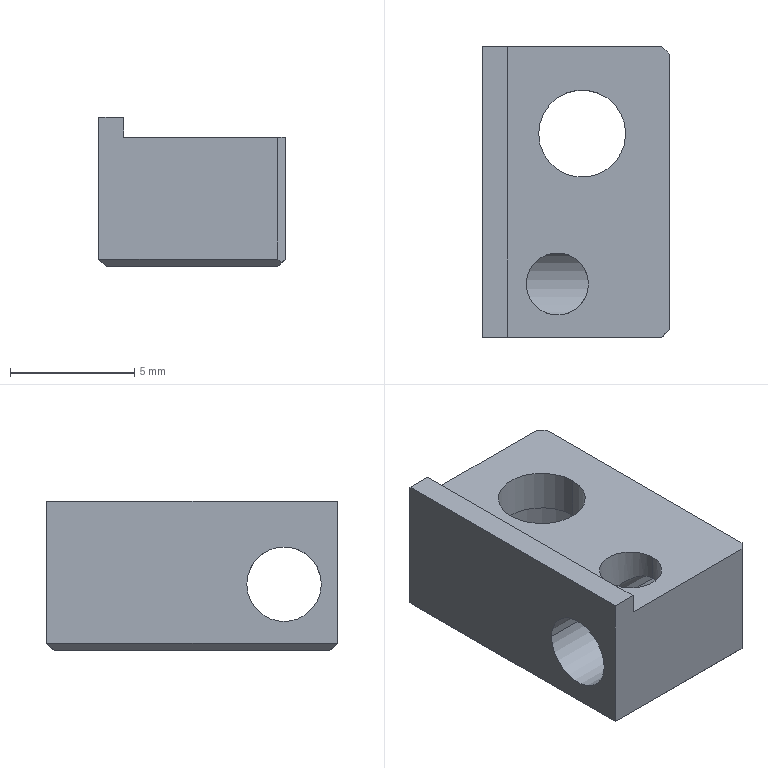Part | NX | 1 solid | 23 faces | box 7.5 x 11.687 x 6 mm | volume 288.906 mm3 | plane 15 | cylinder 8 | commonest cylinder face diameters 2.5 x2 3 x2 3.5 x2 6 x2
STEP:
#1=CARTESIAN_POINT('',(-53.86,-43.177,4.403));
#2=VERTEX_POINT('',#1);
#3=CARTESIAN_POINT('',(-51.36,-43.177,4.403));
#4=VERTEX_POINT('',#3);
#5=CARTESIAN_POINT('',(-52.61,-43.177,4.403));
#6=DIRECTION('',(0.,0.,1.));
#7=DIRECTION('',(1.,0.,0.));
#8=AXIS2_PLACEMENT_3D('',#5,#6,#7);
#9=CIRCLE('',#8,1.25);
#10=EDGE_CURVE('',#2,#4,#9,.T.);
#11=ORIENTED_EDGE('',*,*,#10,.T.);
#12=CARTESIAN_POINT('',(-51.36,-43.177,3.373));
#13=VERTEX_POINT('',#12);
#14=CARTESIAN_POINT('',(-51.36,-43.177,5.403));
#15=DIRECTION('',(0.,0.,1.));
#16=VECTOR('',#15,1000.);
#17=LINE('',#14,#16);
#18=EDGE_CURVE('',#13,#4,#17,.T.);
#19=ORIENTED_EDGE('',*,*,#18,.F.);
#20=CARTESIAN_POINT('',(-52.61,-44.427,2.702));
#21=VERTEX_POINT('',#20);
#22=CARTESIAN_POINT('',(-52.61,-44.427,2.702));
#23=CARTESIAN_POINT('',(-52.599,-44.427,2.702));
#24=CARTESIAN_POINT('',(-52.588,-44.426,2.702));
#25=CARTESIAN_POINT('',(-52.578,-44.426,2.703));
#26=CARTESIAN_POINT('',(-52.567,-44.426,2.703));
#27=CARTESIAN_POINT('',(-52.556,-44.425,2.704));
#28=CARTESIAN_POINT('',(-52.545,-44.425,2.705));
#29=CARTESIAN_POINT('',(-52.534,-44.424,2.706));
#30=CARTESIAN_POINT('',(-52.523,-44.424,2.707));
#31=CARTESIAN_POINT('',(-52.512,-44.423,2.708));
#32=CARTESIAN_POINT('',(-52.501,-44.422,2.709));
#33=CARTESIAN_POINT('',(-52.491,-44.421,2.711));
#34=CARTESIAN_POINT('',(-52.48,-44.42,2.712));
#35=CARTESIAN_POINT('',(-52.458,-44.418,2.716));
#36=CARTESIAN_POINT('',(-52.437,-44.415,2.72));
#37=CARTESIAN_POINT('',(-52.416,-44.411,2.725));
#38=CARTESIAN_POINT('',(-52.395,-44.408,2.73));
#39=CARTESIAN_POINT('',(-52.374,-44.404,2.735));
#40=CARTESIAN_POINT('',(-52.354,-44.4,2.741));
#41=CARTESIAN_POINT('',(-52.313,-44.391,2.753));
#42=CARTESIAN_POINT('',(-52.273,-44.381,2.768));
#43=CARTESIAN_POINT('',(-52.234,-44.369,2.784));
#44=CARTESIAN_POINT('',(-52.215,-44.363,2.792));
#45=CARTESIAN_POINT('',(-52.196,-44.356,2.8));
#46=CARTESIAN_POINT('',(-52.177,-44.349,2.809));
#47=CARTESIAN_POINT('',(-52.158,-44.342,2.817));
#48=CARTESIAN_POINT('',(-52.139,-44.335,2.826));
#49=CARTESIAN_POINT('',(-52.121,-44.327,2.836));
#50=CARTESIAN_POINT('',(-52.103,-44.319,2.845));
#51=CARTESIAN_POINT('',(-52.085,-44.311,2.854));
#52=CARTESIAN_POINT('',(-52.067,-44.303,2.864));
#53=CARTESIAN_POINT('',(-52.05,-44.294,2.874));
#54=CARTESIAN_POINT('',(-52.033,-44.285,2.884));
#55=CARTESIAN_POINT('',(-52.016,-44.276,2.893));
#56=CARTESIAN_POINT('',(-51.998,-44.267,2.903));
#57=CARTESIAN_POINT('',(-51.982,-44.257,2.913));
#58=CARTESIAN_POINT('',(-51.965,-44.247,2.924));
#59=CARTESIAN_POINT('',(-51.949,-44.237,2.934));
#60=CARTESIAN_POINT('',(-51.932,-44.227,2.944));
#61=CARTESIAN_POINT('',(-51.916,-44.216,2.954));
#62=CARTESIAN_POINT('',(-51.9,-44.205,2.965));
#63=CARTESIAN_POINT('',(-51.884,-44.194,2.975));
#64=CARTESIAN_POINT('',(-51.869,-44.183,2.985));
#65=CARTESIAN_POINT('',(-51.853,-44.171,2.996));
#66=CARTESIAN_POINT('',(-51.838,-44.16,3.006));
#67=CARTESIAN_POINT('',(-51.823,-44.147,3.017));
#68=CARTESIAN_POINT('',(-51.793,-44.123,3.037));
#69=CARTESIAN_POINT('',(-51.764,-44.097,3.058));
#70=CARTESIAN_POINT('',(-51.736,-44.07,3.078));
#71=CARTESIAN_POINT('',(-51.708,-44.043,3.098));
#72=CARTESIAN_POINT('',(-51.682,-44.014,3.118));
#73=CARTESIAN_POINT('',(-51.656,-43.985,3.137));
#74=CARTESIAN_POINT('',(-51.644,-43.97,3.146));
#75=CARTESIAN_POINT('',(-51.631,-43.954,3.156));
#76=CARTESIAN_POINT('',(-51.619,-43.939,3.165));
#77=CARTESIAN_POINT('',(-51.607,-43.923,3.174));
#78=CARTESIAN_POINT('',(-51.596,-43.907,3.183));
#79=CARTESIAN_POINT('',(-51.584,-43.891,3.192));
#80=CARTESIAN_POINT('',(-51.573,-43.874,3.201));
#81=CARTESIAN_POINT('',(-51.562,-43.857,3.21));
#82=CARTESIAN_POINT('',(-51.551,-43.84,3.218));
#83=CARTESIAN_POINT('',(-51.54,-43.823,3.227));
#84=CARTESIAN_POINT('',(-51.53,-43.806,3.235));
#85=CARTESIAN_POINT('',(-51.52,-43.788,3.243));
#86=CARTESIAN_POINT('',(-51.51,-43.77,3.251));
#87=CARTESIAN_POINT('',(-51.5,-43.752,3.259));
#88=CARTESIAN_POINT('',(-51.491,-43.733,3.266));
#89=CARTESIAN_POINT('',(-51.482,-43.715,3.273));
#90=CARTESIAN_POINT('',(-51.473,-43.696,3.28));
#91=CARTESIAN_POINT('',(-51.465,-43.677,3.287));
#92=CARTESIAN_POINT('',(-51.448,-43.639,3.301));
#93=CARTESIAN_POINT('',(-51.433,-43.6,3.313));
#94=CARTESIAN_POINT('',(-51.42,-43.56,3.323));
#95=CARTESIAN_POINT('',(-51.414,-43.539,3.329));
#96=CARTESIAN_POINT('',(-51.408,-43.519,3.334));
#97=CARTESIAN_POINT('',(-51.402,-43.498,3.338));
#98=CARTESIAN_POINT('',(-51.397,-43.478,3.343));
#99=CARTESIAN_POINT('',(-51.392,-43.457,3.347));
#100=CARTESIAN_POINT('',(-51.387,-43.436,3.351));
#101=CARTESIAN_POINT('',(-51.383,-43.414,3.354));
#102=CARTESIAN_POINT('',(-51.379,-43.393,3.358));
#103=CARTESIAN_POINT('',(-51.376,-43.372,3.36));
#104=CARTESIAN_POINT('',(-51.372,-43.35,3.363));
#105=CARTESIAN_POINT('',(-51.369,-43.329,3.366));
#106=CARTESIAN_POINT('',(-51.367,-43.307,3.367));
#107=CARTESIAN_POINT('',(-51.365,-43.285,3.369));
#108=CARTESIAN_POINT('',(-51.363,-43.264,3.371));
#109=CARTESIAN_POINT('',(-51.362,-43.242,3.372));
#110=CARTESIAN_POINT('',(-51.361,-43.22,3.373));
#111=CARTESIAN_POINT('',(-51.36,-43.198,3.373));
#112=CARTESIAN_POINT('',(-51.36,-43.177,3.373));
#113=B_SPLINE_CURVE_WITH_KNOTS('',3,(#22,#23,#24,#25,#26,#27,#28,#29,#30,#31,#32,#33,#34,#35,#36,#37,#38,#39,#40,#41,#42,#43,#44,#45,#46,#47,#48,#49,#50,#51,#52,#53,#54,#55,#56,#57,#58,#59,#60,#61,#62,#63,#64,#65,#66,#67,#68,#69,#70,#71,#72,#73,#74,#75,#76,#77,#78,#79,#80,#81,#82,#83,#84,#85,#86,#87,#88,#89,#90,#91,#92,#93,#94,#95,#96,#97,#98,#99,#100,#101,#102,#103,#104,#105,#106,#107,#108,#109,#110,#111,#112),.UNSPECIFIED.,.F.,.F.,(4,3,3,3,3,3,3,3,3,3,3,3,3,3,3,3,3,3,3,3,3,3,3,3,3,3,3,3,3,3,4),(0.,0.03265,0.06539,0.0982,0.1311,0.1968,0.2623,0.393,0.4586,0.5242,0.5897,0.655,0.7204,0.786,0.8518,0.9176,1.049,1.18,1.245,1.311,1.377,1.442,1.508,1.574,1.705,1.77,1.836,1.902,1.967,2.033,2.098),.UNSPECIFIED.);
#114=EDGE_CURVE('',#21,#13,#113,.T.);
#115=ORIENTED_EDGE('',*,*,#114,.F.);
#116=CARTESIAN_POINT('',(-53.86,-43.177,3.373));
#117=VERTEX_POINT('',#116);
#118=CARTESIAN_POINT('',(-53.86,-43.177,3.373));
#119=CARTESIAN_POINT('',(-53.86,-43.199,3.373));
#120=CARTESIAN_POINT('',(-53.86,-43.22,3.373));
#121=CARTESIAN_POINT('',(-53.859,-43.242,3.372));
#122=CARTESIAN_POINT('',(-53.857,-43.264,3.371));
#123=CARTESIAN_POINT('',(-53.856,-43.286,3.369));
#124=CARTESIAN_POINT('',(-53.853,-43.307,3.367));
#125=CARTESIAN_POINT('',(-53.851,-43.329,3.365));
#126=CARTESIAN_POINT('',(-53.848,-43.35,3.363));
#127=CARTESIAN_POINT('',(-53.845,-43.372,3.36));
#128=CARTESIAN_POINT('',(-53.842,-43.393,3.358));
#129=CARTESIAN_POINT('',(-53.838,-43.414,3.354));
#130=CARTESIAN_POINT('',(-53.833,-43.435,3.351));
#131=CARTESIAN_POINT('',(-53.829,-43.457,3.347));
#132=CARTESIAN_POINT('',(-53.824,-43.478,3.343));
#133=CARTESIAN_POINT('',(-53.818,-43.498,3.338));
#134=CARTESIAN_POINT('',(-53.813,-43.519,3.334));
#135=CARTESIAN_POINT('',(-53.807,-43.539,3.329));
#136=CARTESIAN_POINT('',(-53.8,-43.56,3.323));
#137=CARTESIAN_POINT('',(-53.794,-43.58,3.318));
#138=CARTESIAN_POINT('',(-53.787,-43.6,3.312));
#139=CARTESIAN_POINT('',(-53.779,-43.619,3.306));
#140=CARTESIAN_POINT('',(-53.772,-43.639,3.3));
#141=CARTESIAN_POINT('',(-53.764,-43.658,3.294));
#142=CARTESIAN_POINT('',(-53.756,-43.677,3.287));
#143=CARTESIAN_POINT('',(-53.747,-43.696,3.28));
#144=CARTESIAN_POINT('',(-53.739,-43.715,3.273));
#145=CARTESIAN_POINT('',(-53.73,-43.733,3.266));
#146=CARTESIAN_POINT('',(-53.72,-43.752,3.259));
#147=CARTESIAN_POINT('',(-53.711,-43.77,3.251));
#148=CARTESIAN_POINT('',(-53.701,-43.788,3.243));
#149=CARTESIAN_POINT('',(-53.691,-43.805,3.235));
#150=CARTESIAN_POINT('',(-53.68,-43.823,3.227));
#151=CARTESIAN_POINT('',(-53.67,-43.84,3.218));
#152=CARTESIAN_POINT('',(-53.659,-43.857,3.21));
#153=CARTESIAN_POINT('',(-53.648,-43.874,3.201));
#154=CARTESIAN_POINT('',(-53.636,-43.89,3.192));
#155=CARTESIAN_POINT('',(-53.625,-43.907,3.183));
#156=CARTESIAN_POINT('',(-53.613,-43.923,3.174));
#157=CARTESIAN_POINT('',(-53.601,-43.939,3.165));
#158=CARTESIAN_POINT('',(-53.589,-43.954,3.156));
#159=CARTESIAN_POINT('',(-53.577,-43.97,3.146));
#160=CARTESIAN_POINT('',(-53.564,-43.985,3.137));
#161=CARTESIAN_POINT('',(-53.539,-44.014,3.118));
#162=CARTESIAN_POINT('',(-53.512,-44.043,3.098));
#163=CARTESIAN_POINT('',(-53.485,-44.07,3.078));
#164=CARTESIAN_POINT('',(-53.457,-44.097,3.058));
#165=CARTESIAN_POINT('',(-53.428,-44.123,3.037));
#166=CARTESIAN_POINT('',(-53.398,-44.147,3.017));
#167=CARTESIAN_POINT('',(-53.383,-44.16,3.006));
#168=CARTESIAN_POINT('',(-53.367,-44.171,2.996));
#169=CARTESIAN_POINT('',(-53.352,-44.183,2.986));
#170=CARTESIAN_POINT('',(-53.336,-44.194,2.975));
#171=CARTESIAN_POINT('',(-53.32,-44.205,2.965));
#172=CARTESIAN_POINT('',(-53.304,-44.216,2.954));
#173=CARTESIAN_POINT('',(-53.288,-44.227,2.944));
#174=CARTESIAN_POINT('',(-53.272,-44.237,2.934));
#175=CARTESIAN_POINT('',(-53.255,-44.247,2.924));
#176=CARTESIAN_POINT('',(-53.239,-44.257,2.913));
#177=CARTESIAN_POINT('',(-53.222,-44.267,2.903));
#178=CARTESIAN_POINT('',(-53.205,-44.276,2.893));
#179=CARTESIAN_POINT('',(-53.188,-44.285,2.884));
#180=CARTESIAN_POINT('',(-53.171,-44.294,2.874));
#181=CARTESIAN_POINT('',(-53.153,-44.303,2.864));
#182=CARTESIAN_POINT('',(-53.135,-44.311,2.854));
#183=CARTESIAN_POINT('',(-53.117,-44.319,2.845));
#184=CARTESIAN_POINT('',(-53.099,-44.327,2.836));
#185=CARTESIAN_POINT('',(-53.081,-44.335,2.826));
#186=CARTESIAN_POINT('',(-53.063,-44.342,2.817));
#187=CARTESIAN_POINT('',(-53.044,-44.349,2.809));
#188=CARTESIAN_POINT('',(-53.025,-44.356,2.8));
#189=CARTESIAN_POINT('',(-53.006,-44.363,2.792));
#190=CARTESIAN_POINT('',(-52.986,-44.369,2.784));
#191=CARTESIAN_POINT('',(-52.948,-44.381,2.768));
#192=CARTESIAN_POINT('',(-52.908,-44.391,2.753));
#193=CARTESIAN_POINT('',(-52.867,-44.4,2.741));
#194=CARTESIAN_POINT('',(-52.846,-44.404,2.735));
#195=CARTESIAN_POINT('',(-52.826,-44.408,2.729));
#196=CARTESIAN_POINT('',(-52.804,-44.411,2.725));
#197=CARTESIAN_POINT('',(-52.783,-44.415,2.72));
#198=CARTESIAN_POINT('',(-52.762,-44.418,2.716));
#199=CARTESIAN_POINT('',(-52.74,-44.42,2.712));
#200=CARTESIAN_POINT('',(-52.73,-44.421,2.711));
#201=CARTESIAN_POINT('',(-52.719,-44.422,2.709));
#202=CARTESIAN_POINT('',(-52.708,-44.423,2.708));
#203=CARTESIAN_POINT('',(-52.697,-44.424,2.707));
#204=CARTESIAN_POINT('',(-52.686,-44.424,2.706));
#205=CARTESIAN_POINT('',(-52.675,-44.425,2.705));
#206=CARTESIAN_POINT('',(-52.665,-44.426,2.704));
#207=CARTESIAN_POINT('',(-52.654,-44.426,2.703));
#208=CARTESIAN_POINT('',(-52.643,-44.426,2.703));
#209=CARTESIAN_POINT('',(-52.632,-44.426,2.702));
#210=CARTESIAN_POINT('',(-52.621,-44.427,2.702));
#211=CARTESIAN_POINT('',(-52.61,-44.427,2.702));
#212=B_SPLINE_CURVE_WITH_KNOTS('',3,(#118,#119,#120,#121,#122,#123,#124,#125,#126,#127,#128,#129,#130,#131,#132,#133,#134,#135,#136,#137,#138,#139,#140,#141,#142,#143,#144,#145,#146,#147,#148,#149,#150,#151,#152,#153,#154,#155,#156,#157,#158,#159,#160,#161,#162,#163,#164,#165,#166,#167,#168,#169,#170,#171,#172,#173,#174,#175,#176,#177,#178,#179,#180,#181,#182,#183,#184,#185,#186,#187,#188,#189,#190,#191,#192,#193,#194,#195,#196,#197,#198,#199,#200,#201,#202,#203,#204,#205,#206,#207,#208,#209,#210,#211),.UNSPECIFIED.,.F.,.F.,(4,3,3,3,3,3,3,3,3,3,3,3,3,3,3,3,3,3,3,3,3,3,3,3,3,3,3,3,3,3,3,4),(0.,0.06564,0.131,0.1964,0.262,0.3277,0.3934,0.4588,0.5241,0.5897,0.6553,0.7211,0.7868,0.8525,0.9179,1.049,1.18,1.246,1.312,1.378,1.443,1.508,1.574,1.639,1.705,1.836,1.901,1.967,2.,2.033,2.065,2.098),.UNSPECIFIED.);
#213=EDGE_CURVE('',#117,#21,#212,.T.);
#214=ORIENTED_EDGE('',*,*,#213,.F.);
#215=CARTESIAN_POINT('',(-53.86,-43.177,5.403));
#216=DIRECTION('',(0.,0.,1.));
#217=VECTOR('',#216,1000.);
#218=LINE('',#215,#217);
#219=EDGE_CURVE('',#117,#2,#218,.T.);
#220=ORIENTED_EDGE('',*,*,#219,.T.);
#221=EDGE_LOOP('',(#11,#19,#115,#214,#220));
#222=FACE_BOUND('',#221,.T.);
#223=CARTESIAN_POINT('',(-52.61,-43.177,5.403));
#224=DIRECTION('',(0.,0.,1.));
#225=DIRECTION('',(1.,0.,0.));
#226=AXIS2_PLACEMENT_3D('',#223,#224,#225);
#227=CYLINDRICAL_SURFACE('',#226,1.25);
#228=ADVANCED_FACE('',(#222),#227,.F.);
#229=CARTESIAN_POINT('',(-55.61,-45.316,-0.4969));
#230=VERTEX_POINT('',#229);
#231=CARTESIAN_POINT('',(-55.61,-45.316,5.203));
#232=VERTEX_POINT('',#231);
#233=CARTESIAN_POINT('',(-55.61,-45.316,4.403));
#234=DIRECTION('',(0.,0.,1.));
#235=VECTOR('',#234,1000.);
#236=LINE('',#233,#235);
#237=EDGE_CURVE('',#230,#232,#236,.T.);
#238=ORIENTED_EDGE('',*,*,#237,.T.);
#239=CARTESIAN_POINT('',(-55.61,-33.629,5.203));
#240=VERTEX_POINT('',#239);
#241=CARTESIAN_POINT('',(-55.61,-45.316,5.203));
#242=DIRECTION('',(0.,1.,0.));
#243=VECTOR('',#242,1000.);
#244=LINE('',#241,#243);
#245=EDGE_CURVE('',#232,#240,#244,.T.);
#246=ORIENTED_EDGE('',*,*,#245,.T.);
#247=CARTESIAN_POINT('',(-55.61,-33.629,-0.4969));
#248=VERTEX_POINT('',#247);
#249=CARTESIAN_POINT('',(-55.61,-33.629,4.403));
#250=DIRECTION('',(0.,0.,1.));
#251=VECTOR('',#250,1000.);
#252=LINE('',#249,#251);
#253=EDGE_CURVE('',#248,#240,#252,.T.);
#254=ORIENTED_EDGE('',*,*,#253,.F.);
#255=CARTESIAN_POINT('',(-55.61,-39.622,-0.4969));
#256=DIRECTION('',(0.,1.,0.));
#257=VECTOR('',#256,1000.);
#258=LINE('',#255,#257);
#259=EDGE_CURVE('',#230,#248,#258,.T.);
#260=ORIENTED_EDGE('',*,*,#259,.F.);
#261=EDGE_LOOP('',(#238,#246,#254,#260));
#262=FACE_BOUND('',#261,.T.);
#263=CARTESIAN_POINT('',(-55.61,-41.677,1.873));
#264=VERTEX_POINT('',#263);
#265=CARTESIAN_POINT('',(-55.61,-44.677,1.873));
#266=VERTEX_POINT('',#265);
#267=CARTESIAN_POINT('',(-55.61,-43.177,1.873));
#268=DIRECTION('',(-1.,0.,0.));
#269=DIRECTION('',(0.,-1.,0.));
#270=AXIS2_PLACEMENT_3D('',#267,#268,#269);
#271=CIRCLE('',#270,1.5);
#272=EDGE_CURVE('',#264,#266,#271,.T.);
#273=ORIENTED_EDGE('',*,*,#272,.F.);
#274=CARTESIAN_POINT('',(-55.61,-43.177,1.873));
#275=DIRECTION('',(-1.,0.,0.));
#276=DIRECTION('',(0.,-1.,0.));
#277=AXIS2_PLACEMENT_3D('',#274,#275,#276);
#278=CIRCLE('',#277,1.5);
#279=EDGE_CURVE('',#266,#264,#278,.T.);
#280=ORIENTED_EDGE('',*,*,#279,.F.);
#281=EDGE_LOOP('',(#273,#280));
#282=FACE_BOUND('',#281,.T.);
#283=CARTESIAN_POINT('',(-55.61,-32.629,3.403));
#284=DIRECTION('',(-1.,0.,0.));
#285=DIRECTION('',(0.,0.,1.));
#286=AXIS2_PLACEMENT_3D('',#283,#284,#285);
#287=PLANE('',#286);
#288=ADVANCED_FACE('',(#262,#282),#287,.T.);
#289=ORIENTED_EDGE('',*,*,#253,.T.);
#290=CARTESIAN_POINT('',(-54.61,-33.629,5.203));
#291=VERTEX_POINT('',#290);
#292=CARTESIAN_POINT('',(-55.61,-33.629,5.203));
#293=DIRECTION('',(1.,0.,0.));
#294=VECTOR('',#293,1000.);
#295=LINE('',#292,#294);
#296=EDGE_CURVE('',#240,#291,#295,.T.);
#297=ORIENTED_EDGE('',*,*,#296,.T.);
#298=CARTESIAN_POINT('',(-54.61,-33.629,4.403));
#299=VERTEX_POINT('',#298);
#300=CARTESIAN_POINT('',(-54.61,-33.629,4.403));
#301=DIRECTION('',(0.,0.,1.));
#302=VECTOR('',#301,1000.);
#303=LINE('',#300,#302);
#304=EDGE_CURVE('',#299,#291,#303,.T.);
#305=ORIENTED_EDGE('',*,*,#304,.F.);
#306=CARTESIAN_POINT('',(-48.41,-33.629,4.403));
#307=VERTEX_POINT('',#306);
#308=CARTESIAN_POINT('',(-49.386,-33.629,4.403));
#309=DIRECTION('',(-1.,0.,0.));
#310=VECTOR('',#309,1000.);
#311=LINE('',#308,#310);
#312=EDGE_CURVE('',#307,#299,#311,.T.);
#313=ORIENTED_EDGE('',*,*,#312,.F.);
#314=CARTESIAN_POINT('',(-48.41,-33.629,-0.4969));
#315=VERTEX_POINT('',#314);
#316=CARTESIAN_POINT('',(-48.41,-33.629,1.953));
#317=DIRECTION('',(0.,0.,-1.));
#318=VECTOR('',#317,1000.);
#319=LINE('',#316,#318);
#320=EDGE_CURVE('',#307,#315,#319,.T.);
#321=ORIENTED_EDGE('',*,*,#320,.T.);
#322=CARTESIAN_POINT('',(-52.01,-33.629,-0.4969));
#323=DIRECTION('',(1.,0.,0.));
#324=VECTOR('',#323,1000.);
#325=LINE('',#322,#324);
#326=EDGE_CURVE('',#248,#315,#325,.T.);
#327=ORIENTED_EDGE('',*,*,#326,.F.);
#328=EDGE_LOOP('',(#289,#297,#305,#313,#321,#327));
#329=FACE_BOUND('',#328,.T.);
#330=CARTESIAN_POINT('',(-48.11,-33.629,3.403));
#331=DIRECTION('',(0.,1.,0.));
#332=DIRECTION('',(0.,0.,-1.));
#333=AXIS2_PLACEMENT_3D('',#330,#331,#332);
#334=PLANE('',#333);
#335=ADVANCED_FACE('',(#329),#334,.T.);
#336=CARTESIAN_POINT('',(-48.11,-45.016,4.403));
#337=VERTEX_POINT('',#336);
#338=CARTESIAN_POINT('',(-48.11,-33.929,4.403));
#339=VERTEX_POINT('',#338);
#340=CARTESIAN_POINT('',(-48.11,-36.078,4.403));
#341=DIRECTION('',(0.,1.,0.));
#342=VECTOR('',#341,1000.);
#343=LINE('',#340,#342);
#344=EDGE_CURVE('',#337,#339,#343,.T.);
#345=ORIENTED_EDGE('',*,*,#344,.F.);
#346=CARTESIAN_POINT('',(-48.11,-45.016,-0.4969));
#347=VERTEX_POINT('',#346);
#348=CARTESIAN_POINT('',(-48.11,-45.016,1.953));
#349=DIRECTION('',(0.,0.,1.));
#350=VECTOR('',#349,1000.);
#351=LINE('',#348,#350);
#352=EDGE_CURVE('',#347,#337,#351,.T.);
#353=ORIENTED_EDGE('',*,*,#352,.F.);
#354=CARTESIAN_POINT('',(-48.11,-33.929,-0.4969));
#355=VERTEX_POINT('',#354);
#356=CARTESIAN_POINT('',(-48.11,-36.078,-0.4969));
#357=DIRECTION('',(0.,1.,0.));
#358=VECTOR('',#357,1000.);
#359=LINE('',#356,#358);
#360=EDGE_CURVE('',#347,#355,#359,.T.);
#361=ORIENTED_EDGE('',*,*,#360,.T.);
#362=CARTESIAN_POINT('',(-48.11,-33.929,1.953));
#363=DIRECTION('',(0.,0.,-1.));
#364=VECTOR('',#363,1000.);
#365=LINE('',#362,#364);
#366=EDGE_CURVE('',#339,#355,#365,.T.);
#367=ORIENTED_EDGE('',*,*,#366,.F.);
#368=EDGE_LOOP('',(#345,#353,#361,#367));
#369=FACE_BOUND('',#368,.T.);
#370=CARTESIAN_POINT('',(-48.11,-41.677,1.873));
#371=VERTEX_POINT('',#370);
#372=CARTESIAN_POINT('',(-48.11,-44.677,1.873));
#373=VERTEX_POINT('',#372);
#374=CARTESIAN_POINT('',(-48.11,-43.177,1.873));
#375=DIRECTION('',(-1.,0.,0.));
#376=DIRECTION('',(0.,-1.,0.));
#377=AXIS2_PLACEMENT_3D('',#374,#375,#376);
#378=CIRCLE('',#377,1.5);
#379=EDGE_CURVE('',#371,#373,#378,.T.);
#380=ORIENTED_EDGE('',*,*,#379,.T.);
#381=CARTESIAN_POINT('',(-48.11,-43.177,1.873));
#382=DIRECTION('',(-1.,0.,0.));
#383=DIRECTION('',(0.,-1.,0.));
#384=AXIS2_PLACEMENT_3D('',#381,#382,#383);
#385=CIRCLE('',#384,1.5);
#386=EDGE_CURVE('',#373,#371,#385,.T.);
#387=ORIENTED_EDGE('',*,*,#386,.T.);
#388=EDGE_LOOP('',(#380,#387));
#389=FACE_BOUND('',#388,.T.);
#390=CARTESIAN_POINT('',(-48.11,-52.629,3.403));
#391=DIRECTION('',(1.,0.,0.));
#392=DIRECTION('',(0.,0.,1.));
#393=AXIS2_PLACEMENT_3D('',#390,#391,#392);
#394=PLANE('',#393);
#395=ADVANCED_FACE('',(#369,#389),#394,.T.);
#396=ORIENTED_EDGE('',*,*,#379,.F.);
#397=CARTESIAN_POINT('',(-47.41,-41.677,1.873));
#398=DIRECTION('',(-1.,0.,0.));
#399=VECTOR('',#398,1000.);
#400=LINE('',#397,#399);
#401=EDGE_CURVE('',#264,#371,#400,.F.);
#402=ORIENTED_EDGE('',*,*,#401,.F.);
#403=ORIENTED_EDGE('',*,*,#272,.T.);
#404=CARTESIAN_POINT('',(-47.41,-44.677,1.873));
#405=DIRECTION('',(-1.,0.,0.));
#406=VECTOR('',#405,1000.);
#407=LINE('',#404,#406);
#408=EDGE_CURVE('',#266,#373,#407,.F.);
#409=ORIENTED_EDGE('',*,*,#408,.T.);
#410=EDGE_LOOP('',(#396,#402,#403,#409));
#411=FACE_BOUND('',#410,.T.);
#412=CARTESIAN_POINT('',(-47.41,-43.177,1.873));
#413=DIRECTION('',(-1.,0.,0.));
#414=DIRECTION('',(0.,-1.,0.));
#415=AXIS2_PLACEMENT_3D('',#412,#413,#414);
#416=CYLINDRICAL_SURFACE('',#415,1.5);
#417=ADVANCED_FACE('',(#411),#416,.F.);
#418=ORIENTED_EDGE('',*,*,#320,.F.);
#419=CARTESIAN_POINT('',(-49.386,-32.653,4.403));
#420=DIRECTION('',(-0.7071,0.7071,0.));
#421=VECTOR('',#420,1000.);
#422=LINE('',#419,#421);
#423=EDGE_CURVE('',#339,#307,#422,.T.);
#424=ORIENTED_EDGE('',*,*,#423,.F.);
#425=ORIENTED_EDGE('',*,*,#366,.T.);
#426=CARTESIAN_POINT('',(-48.26,-33.779,-0.6469));
#427=VERTEX_POINT('',#426);
#428=CARTESIAN_POINT('',(-49.386,-32.653,-1.773));
#429=DIRECTION('',(0.5774,-0.5774,0.5774));
#430=VECTOR('',#429,1000.);
#431=LINE('',#428,#430);
#432=EDGE_CURVE('',#427,#355,#431,.T.);
#433=ORIENTED_EDGE('',*,*,#432,.F.);
#434=CARTESIAN_POINT('',(-49.386,-32.653,0.4788));
#435=DIRECTION('',(0.5774,-0.5774,-0.5774));
#436=VECTOR('',#435,1000.);
#437=LINE('',#434,#436);
#438=EDGE_CURVE('',#315,#427,#437,.T.);
#439=ORIENTED_EDGE('',*,*,#438,.F.);
#440=EDGE_LOOP('',(#418,#424,#425,#433,#439));
#441=FACE_BOUND('',#440,.T.);
#442=CARTESIAN_POINT('',(-48.26,-33.779,1.953));
#443=DIRECTION('',(0.7071,0.7071,0.));
#444=DIRECTION('',(0.,0.,-1.));
#445=AXIS2_PLACEMENT_3D('',#442,#443,#444);
#446=PLANE('',#445);
#447=ADVANCED_FACE('',(#441),#446,.T.);
#448=ORIENTED_EDGE('',*,*,#245,.F.);
#449=CARTESIAN_POINT('',(-54.61,-45.316,5.203));
#450=VERTEX_POINT('',#449);
#451=CARTESIAN_POINT('',(-54.61,-45.316,5.203));
#452=DIRECTION('',(-1.,0.,0.));
#453=VECTOR('',#452,1000.);
#454=LINE('',#451,#453);
#455=EDGE_CURVE('',#450,#232,#454,.T.);
#456=ORIENTED_EDGE('',*,*,#455,.F.);
#457=CARTESIAN_POINT('',(-54.61,-33.629,5.203));
#458=DIRECTION('',(0.,-1.,0.));
#459=VECTOR('',#458,1000.);
#460=LINE('',#457,#459);
#461=EDGE_CURVE('',#291,#450,#460,.T.);
#462=ORIENTED_EDGE('',*,*,#461,.F.);
#463=ORIENTED_EDGE('',*,*,#296,.F.);
#464=EDGE_LOOP('',(#448,#456,#462,#463));
#465=FACE_BOUND('',#464,.T.);
#466=CARTESIAN_POINT('',(-54.321,-38.07,5.203));
#467=DIRECTION('',(0.,0.,1.));
#468=DIRECTION('',(1.,0.,0.));
#469=AXIS2_PLACEMENT_3D('',#466,#467,#468);
#470=PLANE('',#469);
#471=ADVANCED_FACE('',(#465),#470,.T.);
#472=CARTESIAN_POINT('',(-54.61,-45.316,4.403));
#473=VERTEX_POINT('',#472);
#474=CARTESIAN_POINT('',(-54.61,-36.078,4.403));
#475=DIRECTION('',(0.,-1.,0.));
#476=VECTOR('',#475,1000.);
#477=LINE('',#474,#476);
#478=EDGE_CURVE('',#299,#473,#477,.T.);
#479=ORIENTED_EDGE('',*,*,#478,.F.);
#480=ORIENTED_EDGE('',*,*,#304,.T.);
#481=ORIENTED_EDGE('',*,*,#461,.T.);
#482=CARTESIAN_POINT('',(-54.61,-45.316,4.403));
#483=DIRECTION('',(0.,0.,1.));
#484=VECTOR('',#483,1000.);
#485=LINE('',#482,#484);
#486=EDGE_CURVE('',#473,#450,#485,.T.);
#487=ORIENTED_EDGE('',*,*,#486,.F.);
#488=EDGE_LOOP('',(#479,#480,#481,#487));
#489=FACE_BOUND('',#488,.T.);
#490=CARTESIAN_POINT('',(-54.61,-33.629,4.403));
#491=DIRECTION('',(1.,0.,0.));
#492=DIRECTION('',(0.,1.,0.));
#493=AXIS2_PLACEMENT_3D('',#490,#491,#492);
#494=PLANE('',#493);
#495=ADVANCED_FACE('',(#489),#494,.T.);
#496=ORIENTED_EDGE('',*,*,#18,.T.);
#497=CARTESIAN_POINT('',(-52.61,-43.177,4.403));
#498=DIRECTION('',(0.,0.,1.));
#499=DIRECTION('',(1.,0.,0.));
#500=AXIS2_PLACEMENT_3D('',#497,#498,#499);
#501=CIRCLE('',#500,1.25);
#502=EDGE_CURVE('',#4,#2,#501,.T.);
#503=ORIENTED_EDGE('',*,*,#502,.T.);
#504=ORIENTED_EDGE('',*,*,#219,.F.);
#505=CARTESIAN_POINT('',(-51.36,-43.177,3.373));
#506=CARTESIAN_POINT('',(-51.36,-43.148,3.373));
#507=CARTESIAN_POINT('',(-51.361,-43.12,3.372));
#508=CARTESIAN_POINT('',(-51.363,-43.092,3.371));
#509=CARTESIAN_POINT('',(-51.364,-43.077,3.37));
#510=CARTESIAN_POINT('',(-51.365,-43.062,3.369));
#511=CARTESIAN_POINT('',(-51.367,-43.047,3.367));
#512=CARTESIAN_POINT('',(-51.369,-43.032,3.366));
#513=CARTESIAN_POINT('',(-51.37,-43.017,3.365));
#514=CARTESIAN_POINT('',(-51.373,-43.002,3.363));
#515=CARTESIAN_POINT('',(-51.375,-42.987,3.361));
#516=CARTESIAN_POINT('',(-51.377,-42.972,3.359));
#517=CARTESIAN_POINT('',(-51.38,-42.957,3.357));
#518=CARTESIAN_POINT('',(-51.382,-42.942,3.355));
#519=CARTESIAN_POINT('',(-51.385,-42.928,3.352));
#520=CARTESIAN_POINT('',(-51.388,-42.913,3.35));
#521=CARTESIAN_POINT('',(-51.395,-42.884,3.345));
#522=CARTESIAN_POINT('',(-51.402,-42.855,3.339));
#523=CARTESIAN_POINT('',(-51.41,-42.827,3.332));
#524=CARTESIAN_POINT('',(-51.418,-42.798,3.325));
#525=CARTESIAN_POINT('',(-51.428,-42.771,3.317));
#526=CARTESIAN_POINT('',(-51.438,-42.743,3.309));
#527=CARTESIAN_POINT('',(-51.448,-42.716,3.301));
#528=CARTESIAN_POINT('',(-51.459,-42.689,3.292));
#529=CARTESIAN_POINT('',(-51.471,-42.662,3.282));
#530=CARTESIAN_POINT('',(-51.483,-42.636,3.273));
#531=CARTESIAN_POINT('',(-51.495,-42.611,3.262));
#532=CARTESIAN_POINT('',(-51.509,-42.586,3.252));
#533=CARTESIAN_POINT('',(-51.516,-42.573,3.246));
#534=CARTESIAN_POINT('',(-51.522,-42.561,3.241));
#535=CARTESIAN_POINT('',(-51.529,-42.549,3.235));
#536=CARTESIAN_POINT('',(-51.536,-42.537,3.23));
#537=CARTESIAN_POINT('',(-51.544,-42.525,3.224));
#538=CARTESIAN_POINT('',(-51.551,-42.513,3.218));
#539=CARTESIAN_POINT('',(-51.566,-42.489,3.206));
#540=CARTESIAN_POINT('',(-51.582,-42.466,3.194));
#541=CARTESIAN_POINT('',(-51.598,-42.444,3.182));
#542=CARTESIAN_POINT('',(-51.616,-42.419,3.168));
#543=CARTESIAN_POINT('',(-51.635,-42.394,3.153));
#544=CARTESIAN_POINT('',(-51.654,-42.371,3.138));
#545=CARTESIAN_POINT('',(-51.674,-42.348,3.124));
#546=CARTESIAN_POINT('',(-51.695,-42.325,3.108));
#547=CARTESIAN_POINT('',(-51.716,-42.304,3.093));
#548=CARTESIAN_POINT('',(-51.737,-42.282,3.077));
#549=CARTESIAN_POINT('',(-51.758,-42.261,3.062));
#550=CARTESIAN_POINT('',(-51.781,-42.241,3.046));
#551=CARTESIAN_POINT('',(-51.792,-42.232,3.038));
#552=CARTESIAN_POINT('',(-51.803,-42.222,3.03));
#553=CARTESIAN_POINT('',(-51.815,-42.212,3.022));
#554=CARTESIAN_POINT('',(-51.826,-42.203,3.014));
#555=CARTESIAN_POINT('',(-51.838,-42.194,3.006));
#556=CARTESIAN_POINT('',(-51.85,-42.185,2.998));
#557=CARTESIAN_POINT('',(-51.873,-42.166,2.982));
#558=CARTESIAN_POINT('',(-51.898,-42.149,2.966));
#559=CARTESIAN_POINT('',(-51.923,-42.133,2.95));
#560=CARTESIAN_POINT('',(-51.948,-42.116,2.934));
#561=CARTESIAN_POINT('',(-51.973,-42.101,2.918));
#562=CARTESIAN_POINT('',(-52.,-42.086,2.903));
#563=CARTESIAN_POINT('',(-52.026,-42.071,2.887));
#564=CARTESIAN_POINT('',(-52.053,-42.057,2.872));
#565=CARTESIAN_POINT('',(-52.081,-42.044,2.857));
#566=CARTESIAN_POINT('',(-52.108,-42.032,2.842));
#567=CARTESIAN_POINT('',(-52.136,-42.02,2.828));
#568=CARTESIAN_POINT('',(-52.165,-42.009,2.814));
#569=CARTESIAN_POINT('',(-52.182,-42.002,2.806));
#570=CARTESIAN_POINT('',(-52.199,-41.996,2.799));
#571=CARTESIAN_POINT('',(-52.216,-41.99,2.791));
#572=CARTESIAN_POINT('',(-52.233,-41.985,2.784));
#573=CARTESIAN_POINT('',(-52.251,-41.979,2.777));
#574=CARTESIAN_POINT('',(-52.269,-41.974,2.77));
#575=CARTESIAN_POINT('',(-52.286,-41.969,2.763));
#576=CARTESIAN_POINT('',(-52.304,-41.964,2.757));
#577=CARTESIAN_POINT('',(-52.323,-41.96,2.751));
#578=CARTESIAN_POINT('',(-52.341,-41.956,2.745));
#579=CARTESIAN_POINT('',(-52.36,-41.952,2.739));
#580=CARTESIAN_POINT('',(-52.378,-41.948,2.734));
#581=CARTESIAN_POINT('',(-52.397,-41.945,2.729));
#582=CARTESIAN_POINT('',(-52.416,-41.942,2.725));
#583=CARTESIAN_POINT('',(-52.435,-41.939,2.721));
#584=CARTESIAN_POINT('',(-52.454,-41.936,2.717));
#585=CARTESIAN_POINT('',(-52.473,-41.934,2.713));
#586=CARTESIAN_POINT('',(-52.492,-41.932,2.711));
#587=CARTESIAN_POINT('',(-52.512,-41.93,2.708));
#588=CARTESIAN_POINT('',(-52.531,-41.929,2.706));
#589=CARTESIAN_POINT('',(-52.551,-41.928,2.704));
#590=CARTESIAN_POINT('',(-52.57,-41.927,2.703));
#591=CARTESIAN_POINT('',(-52.59,-41.927,2.702));
#592=CARTESIAN_POINT('',(-52.61,-41.927,2.702));
#593=CARTESIAN_POINT('',(-52.63,-41.927,2.702));
#594=CARTESIAN_POINT('',(-52.649,-41.927,2.703));
#595=CARTESIAN_POINT('',(-52.669,-41.928,2.704));
#596=CARTESIAN_POINT('',(-52.689,-41.929,2.706));
#597=CARTESIAN_POINT('',(-52.708,-41.93,2.708));
#598=CARTESIAN_POINT('',(-52.728,-41.932,2.711));
#599=CARTESIAN_POINT('',(-52.747,-41.934,2.713));
#600=CARTESIAN_POINT('',(-52.766,-41.936,2.717));
#601=CARTESIAN_POINT('',(-52.785,-41.939,2.72));
#602=CARTESIAN_POINT('',(-52.804,-41.942,2.724));
#603=CARTESIAN_POINT('',(-52.823,-41.945,2.729));
#604=CARTESIAN_POINT('',(-52.842,-41.948,2.734));
#605=CARTESIAN_POINT('',(-52.86,-41.952,2.739));
#606=CARTESIAN_POINT('',(-52.879,-41.956,2.744));
#607=CARTESIAN_POINT('',(-52.897,-41.96,2.75));
#608=CARTESIAN_POINT('',(-52.915,-41.964,2.756));
#609=CARTESIAN_POINT('',(-52.933,-41.969,2.763));
#610=CARTESIAN_POINT('',(-52.951,-41.974,2.77));
#611=CARTESIAN_POINT('',(-52.969,-41.979,2.776));
#612=CARTESIAN_POINT('',(-52.987,-41.984,2.783));
#613=CARTESIAN_POINT('',(-53.004,-41.99,2.791));
#614=CARTESIAN_POINT('',(-53.021,-41.996,2.798));
#615=CARTESIAN_POINT('',(-53.038,-42.002,2.806));
#616=CARTESIAN_POINT('',(-53.055,-42.008,2.814));
#617=CARTESIAN_POINT('',(-53.084,-42.019,2.827));
#618=CARTESIAN_POINT('',(-53.112,-42.031,2.842));
#619=CARTESIAN_POINT('',(-53.139,-42.044,2.857));
#620=CARTESIAN_POINT('',(-53.167,-42.057,2.871));
#621=CARTESIAN_POINT('',(-53.194,-42.071,2.887));
#622=CARTESIAN_POINT('',(-53.22,-42.086,2.902));
#623=CARTESIAN_POINT('',(-53.246,-42.1,2.918));
#624=CARTESIAN_POINT('',(-53.272,-42.116,2.934));
#625=CARTESIAN_POINT('',(-53.297,-42.132,2.95));
#626=CARTESIAN_POINT('',(-53.322,-42.149,2.966));
#627=CARTESIAN_POINT('',(-53.346,-42.166,2.982));
#628=CARTESIAN_POINT('',(-53.37,-42.184,2.998));
#629=CARTESIAN_POINT('',(-53.382,-42.193,3.006));
#630=CARTESIAN_POINT('',(-53.394,-42.202,3.014));
#631=CARTESIAN_POINT('',(-53.405,-42.212,3.022));
#632=CARTESIAN_POINT('',(-53.417,-42.221,3.03));
#633=CARTESIAN_POINT('',(-53.428,-42.231,3.038));
#634=CARTESIAN_POINT('',(-53.439,-42.241,3.045));
#635=CARTESIAN_POINT('',(-53.461,-42.261,3.061));
#636=CARTESIAN_POINT('',(-53.483,-42.281,3.077));
#637=CARTESIAN_POINT('',(-53.504,-42.303,3.092));
#638=CARTESIAN_POINT('',(-53.525,-42.325,3.108));
#639=CARTESIAN_POINT('',(-53.546,-42.347,3.123));
#640=CARTESIAN_POINT('',(-53.566,-42.371,3.138));
#641=CARTESIAN_POINT('',(-53.585,-42.394,3.153));
#642=CARTESIAN_POINT('',(-53.604,-42.418,3.167));
#643=CARTESIAN_POINT('',(-53.622,-42.443,3.182));
#644=CARTESIAN_POINT('',(-53.639,-42.466,3.194));
#645=CARTESIAN_POINT('',(-53.654,-42.489,3.206));
#646=CARTESIAN_POINT('',(-53.669,-42.512,3.218));
#647=CARTESIAN_POINT('',(-53.684,-42.536,3.23));
#648=CARTESIAN_POINT('',(-53.698,-42.56,3.241));
#649=CARTESIAN_POINT('',(-53.711,-42.585,3.252));
#650=CARTESIAN_POINT('',(-53.725,-42.61,3.262));
#651=CARTESIAN_POINT('',(-53.737,-42.636,3.272));
#652=CARTESIAN_POINT('',(-53.749,-42.662,3.282));
#653=CARTESIAN_POINT('',(-53.761,-42.688,3.292));
#654=CARTESIAN_POINT('',(-53.772,-42.715,3.301));
#655=CARTESIAN_POINT('',(-53.782,-42.743,3.309));
#656=CARTESIAN_POINT('',(-53.793,-42.77,3.317));
#657=CARTESIAN_POINT('',(-53.802,-42.798,3.325));
#658=CARTESIAN_POINT('',(-53.81,-42.826,3.332));
#659=CARTESIAN_POINT('',(-53.819,-42.855,3.338));
#660=CARTESIAN_POINT('',(-53.826,-42.884,3.345));
#661=CARTESIAN_POINT('',(-53.832,-42.913,3.35));
#662=CARTESIAN_POINT('',(-53.835,-42.928,3.352));
#663=CARTESIAN_POINT('',(-53.838,-42.942,3.355));
#664=CARTESIAN_POINT('',(-53.841,-42.957,3.357));
#665=CARTESIAN_POINT('',(-53.843,-42.972,3.359));
#666=CARTESIAN_POINT('',(-53.846,-42.986,3.361));
#667=CARTESIAN_POINT('',(-53.848,-43.001,3.363));
#668=CARTESIAN_POINT('',(-53.85,-43.016,3.365));
#669=CARTESIAN_POINT('',(-53.852,-43.031,3.366));
#670=CARTESIAN_POINT('',(-53.853,-43.046,3.367));
#671=CARTESIAN_POINT('',(-53.855,-43.061,3.369));
#672=CARTESIAN_POINT('',(-53.856,-43.076,3.37));
#673=CARTESIAN_POINT('',(-53.857,-43.091,3.371));
#674=CARTESIAN_POINT('',(-53.859,-43.12,3.372));
#675=CARTESIAN_POINT('',(-53.86,-43.148,3.373));
#676=CARTESIAN_POINT('',(-53.86,-43.177,3.373));
#677=B_SPLINE_CURVE_WITH_KNOTS('',3,(#505,#506,#507,#508,#509,#510,#511,#512,#513,#514,#515,#516,#517,#518,#519,#520,#521,#522,#523,#524,#525,#526,#527,#528,#529,#530,#531,#532,#533,#534,#535,#536,#537,#538,#539,#540,#541,#542,#543,#544,#545,#546,#547,#548,#549,#550,#551,#552,#553,#554,#555,#556,#557,#558,#559,#560,#561,#562,#563,#564,#565,#566,#567,#568,#569,#570,#571,#572,#573,#574,#575,#576,#577,#578,#579,#580,#581,#582,#583,#584,#585,#586,#587,#588,#589,#590,#591,#592,#593,#594,#595,#596,#597,#598,#599,#600,#601,#602,#603,#604,#605,#606,#607,#608,#609,#610,#611,#612,#613,#614,#615,#616,#617,#618,#619,#620,#621,#622,#623,#624,#625,#626,#627,#628,#629,#630,#631,#632,#633,#634,#635,#636,#637,#638,#639,#640,#641,#642,#643,#644,#645,#646,#647,#648,#649,#650,#651,#652,#653,#654,#655,#656,#657,#658,#659,#660,#661,#662,#663,#664,#665,#666,#667,#668,#669,#670,#671,#672,#673,#674,#675,#676),.UNSPECIFIED.,.F.,.F.,(4,3,3,3,3,3,3,3,3,3,3,3,3,3,3,3,3,3,3,3,3,3,3,3,3,3,3,3,3,3,3,3,3,3,3,3,3,3,3,3,3,3,3,3,3,3,3,3,3,3,3,3,3,3,3,3,3,4),(0.,0.08477,0.1304,0.176,0.2215,0.2669,0.3577,0.4488,0.54,0.631,0.6763,0.7217,0.8127,0.9145,1.016,1.118,1.169,1.219,1.321,1.423,1.524,1.626,1.685,1.744,1.803,1.862,1.921,1.98,2.038,2.098,2.157,2.216,2.275,2.334,2.393,2.452,2.511,2.57,2.671,2.772,2.874,2.976,3.027,3.077,3.179,3.281,3.383,3.474,3.565,3.655,3.747,3.838,3.929,3.974,4.02,4.065,4.111,4.196),.UNSPECIFIED.);
#678=EDGE_CURVE('',#13,#117,#677,.T.);
#679=ORIENTED_EDGE('',*,*,#678,.F.);
#680=EDGE_LOOP('',(#496,#503,#504,#679));
#681=FACE_BOUND('',#680,.T.);
#682=CARTESIAN_POINT('',(-52.61,-43.177,5.403));
#683=DIRECTION('',(0.,0.,1.));
#684=DIRECTION('',(1.,0.,0.));
#685=AXIS2_PLACEMENT_3D('',#682,#683,#684);
#686=CYLINDRICAL_SURFACE('',#685,1.25);
#687=ADVANCED_FACE('',(#681),#686,.F.);
#688=ORIENTED_EDGE('',*,*,#408,.F.);
#689=ORIENTED_EDGE('',*,*,#279,.T.);
#690=ORIENTED_EDGE('',*,*,#401,.T.);
#691=ORIENTED_EDGE('',*,*,#386,.F.);
#692=EDGE_LOOP('',(#688,#689,#690,#691));
#693=FACE_BOUND('',#692,.T.);
#694=ORIENTED_EDGE('',*,*,#213,.T.);
#695=ORIENTED_EDGE('',*,*,#114,.T.);
#696=ORIENTED_EDGE('',*,*,#678,.T.);
#697=EDGE_LOOP('',(#694,#695,#696));
#698=FACE_BOUND('',#697,.T.);
#699=CARTESIAN_POINT('',(-47.41,-43.177,1.873));
#700=DIRECTION('',(-1.,0.,0.));
#701=DIRECTION('',(0.,-1.,0.));
#702=AXIS2_PLACEMENT_3D('',#699,#700,#701);
#703=CYLINDRICAL_SURFACE('',#702,1.5);
#704=ADVANCED_FACE('',(#693,#698),#703,.F.);
#705=CARTESIAN_POINT('',(-55.31,-45.016,-0.7969));
#706=VERTEX_POINT('',#705);
#707=CARTESIAN_POINT('',(-55.31,-33.929,-0.7969));
#708=VERTEX_POINT('',#707);
#709=CARTESIAN_POINT('',(-55.31,-39.622,-0.7969));
#710=DIRECTION('',(0.,1.,0.));
#711=VECTOR('',#710,1000.);
#712=LINE('',#709,#711);
#713=EDGE_CURVE('',#706,#708,#712,.T.);
#714=ORIENTED_EDGE('',*,*,#713,.T.);
#715=CARTESIAN_POINT('',(-48.41,-33.929,-0.7969));
#716=VERTEX_POINT('',#715);
#717=CARTESIAN_POINT('',(-49.386,-33.929,-0.7969));
#718=DIRECTION('',(1.,0.,0.));
#719=VECTOR('',#718,1000.);
#720=LINE('',#717,#719);
#721=EDGE_CURVE('',#708,#716,#720,.T.);
#722=ORIENTED_EDGE('',*,*,#721,.T.);
#723=CARTESIAN_POINT('',(-48.41,-45.016,-0.7969));
#724=VERTEX_POINT('',#723);
#725=CARTESIAN_POINT('',(-48.41,-36.078,-0.7969));
#726=DIRECTION('',(0.,1.,0.));
#727=VECTOR('',#726,1000.);
#728=LINE('',#725,#727);
#729=EDGE_CURVE('',#724,#716,#728,.T.);
#730=ORIENTED_EDGE('',*,*,#729,.F.);
#731=CARTESIAN_POINT('',(-52.01,-45.016,-0.7969));
#732=DIRECTION('',(-1.,0.,0.));
#733=VECTOR('',#732,1000.);
#734=LINE('',#731,#733);
#735=EDGE_CURVE('',#724,#706,#734,.T.);
#736=ORIENTED_EDGE('',*,*,#735,.T.);
#737=EDGE_LOOP('',(#714,#722,#730,#736));
#738=FACE_BOUND('',#737,.T.);
#739=CARTESIAN_POINT('',(-48.61,-37.129,-0.7969));
#740=VERTEX_POINT('',#739);
#741=CARTESIAN_POINT('',(-54.61,-37.129,-0.7969));
#742=VERTEX_POINT('',#741);
#743=CARTESIAN_POINT('',(-51.61,-37.129,-0.7969));
#744=DIRECTION('',(0.,0.,-1.));
#745=DIRECTION('',(-1.,0.,0.));
#746=AXIS2_PLACEMENT_3D('',#743,#744,#745);
#747=CIRCLE('',#746,3.);
#748=EDGE_CURVE('',#740,#742,#747,.T.);
#749=ORIENTED_EDGE('',*,*,#748,.F.);
#750=CARTESIAN_POINT('',(-51.61,-37.129,-0.7969));
#751=DIRECTION('',(0.,0.,-1.));
#752=DIRECTION('',(-1.,0.,0.));
#753=AXIS2_PLACEMENT_3D('',#750,#751,#752);
#754=CIRCLE('',#753,3.);
#755=EDGE_CURVE('',#742,#740,#754,.T.);
#756=ORIENTED_EDGE('',*,*,#755,.F.);
#757=EDGE_LOOP('',(#749,#756));
#758=FACE_BOUND('',#757,.T.);
#759=CARTESIAN_POINT('',(-49.386,-36.078,-0.7969));
#760=DIRECTION('',(0.,0.,-1.));
#761=DIRECTION('',(0.,-1.,0.));
#762=AXIS2_PLACEMENT_3D('',#759,#760,#761);
#763=PLANE('',#762);
#764=ADVANCED_FACE('',(#738,#758),#763,.T.);
#765=CARTESIAN_POINT('',(-48.41,-45.316,-0.4969));
#766=VERTEX_POINT('',#765);
#767=CARTESIAN_POINT('',(-52.01,-45.316,-0.4969));
#768=DIRECTION('',(-1.,0.,0.));
#769=VECTOR('',#768,1000.);
#770=LINE('',#767,#769);
#771=EDGE_CURVE('',#766,#230,#770,.T.);
#772=ORIENTED_EDGE('',*,*,#771,.F.);
#773=CARTESIAN_POINT('',(-48.41,-45.316,4.403));
#774=VERTEX_POINT('',#773);
#775=CARTESIAN_POINT('',(-48.41,-45.316,1.953));
#776=DIRECTION('',(0.,0.,1.));
#777=VECTOR('',#776,1000.);
#778=LINE('',#775,#777);
#779=EDGE_CURVE('',#766,#774,#778,.T.);
#780=ORIENTED_EDGE('',*,*,#779,.T.);
#781=CARTESIAN_POINT('',(-49.386,-45.316,4.403));
#782=DIRECTION('',(-1.,0.,0.));
#783=VECTOR('',#782,1000.);
#784=LINE('',#781,#783);
#785=EDGE_CURVE('',#774,#473,#784,.T.);
#786=ORIENTED_EDGE('',*,*,#785,.T.);
#787=ORIENTED_EDGE('',*,*,#486,.T.);
#788=ORIENTED_EDGE('',*,*,#455,.T.);
#789=ORIENTED_EDGE('',*,*,#237,.F.);
#790=EDGE_LOOP('',(#772,#780,#786,#787,#788,#789));
#791=FACE_BOUND('',#790,.T.);
#792=CARTESIAN_POINT('',(-33.55,-45.316,3.403));
#793=DIRECTION('',(0.,-1.,0.));
#794=DIRECTION('',(-1.,0.,0.));
#795=AXIS2_PLACEMENT_3D('',#792,#793,#794);
#796=PLANE('',#795);
#797=ADVANCED_FACE('',(#791),#796,.T.);
#798=ORIENTED_EDGE('',*,*,#478,.T.);
#799=ORIENTED_EDGE('',*,*,#785,.F.);
#800=CARTESIAN_POINT('',(-49.386,-46.292,4.403));
#801=DIRECTION('',(0.7071,0.7071,0.));
#802=VECTOR('',#801,1000.);
#803=LINE('',#800,#802);
#804=EDGE_CURVE('',#774,#337,#803,.T.);
#805=ORIENTED_EDGE('',*,*,#804,.T.);
#806=ORIENTED_EDGE('',*,*,#344,.T.);
#807=ORIENTED_EDGE('',*,*,#423,.T.);
#808=ORIENTED_EDGE('',*,*,#312,.T.);
#809=EDGE_LOOP('',(#798,#799,#805,#806,#807,#808));
#810=FACE_BOUND('',#809,.T.);
#811=CARTESIAN_POINT('',(-49.86,-37.129,4.403));
#812=VERTEX_POINT('',#811);
#813=CARTESIAN_POINT('',(-53.36,-37.129,4.403));
#814=VERTEX_POINT('',#813);
#815=CARTESIAN_POINT('',(-51.61,-37.129,4.403));
#816=DIRECTION('',(0.,0.,-1.));
#817=DIRECTION('',(-1.,0.,0.));
#818=AXIS2_PLACEMENT_3D('',#815,#816,#817);
#819=CIRCLE('',#818,1.75);
#820=EDGE_CURVE('',#812,#814,#819,.T.);
#821=ORIENTED_EDGE('',*,*,#820,.T.);
#822=CARTESIAN_POINT('',(-51.61,-37.129,4.403));
#823=DIRECTION('',(0.,0.,-1.));
#824=DIRECTION('',(-1.,0.,0.));
#825=AXIS2_PLACEMENT_3D('',#822,#823,#824);
#826=CIRCLE('',#825,1.75);
#827=EDGE_CURVE('',#814,#812,#826,.T.);
#828=ORIENTED_EDGE('',*,*,#827,.T.);
#829=EDGE_LOOP('',(#821,#828));
#830=FACE_BOUND('',#829,.T.);
#831=ORIENTED_EDGE('',*,*,#10,.F.);
#832=ORIENTED_EDGE('',*,*,#502,.F.);
#833=EDGE_LOOP('',(#831,#832));
#834=FACE_BOUND('',#833,.T.);
#835=CARTESIAN_POINT('',(-49.386,-36.078,4.403));
#836=DIRECTION('',(0.,0.,-1.));
#837=DIRECTION('',(0.,-1.,0.));
#838=AXIS2_PLACEMENT_3D('',#835,#836,#837);
#839=PLANE('',#838);
#840=ADVANCED_FACE('',(#810,#830,#834),#839,.F.);
#841=CARTESIAN_POINT('',(-53.161,-36.078,-2.946));
#842=DIRECTION('',(0.5774,-0.5774,-0.5774));
#843=VECTOR('',#842,1000.);
#844=LINE('',#841,#843);
#845=EDGE_CURVE('',#248,#708,#844,.T.);
#846=ORIENTED_EDGE('',*,*,#845,.F.);
#847=ORIENTED_EDGE('',*,*,#326,.T.);
#848=ORIENTED_EDGE('',*,*,#438,.T.);
#849=CARTESIAN_POINT('',(-49.386,-34.905,-1.773));
#850=DIRECTION('',(0.5774,0.5774,0.5774));
#851=VECTOR('',#850,1000.);
#852=LINE('',#849,#851);
#853=EDGE_CURVE('',#716,#427,#852,.T.);
#854=ORIENTED_EDGE('',*,*,#853,.F.);
#855=ORIENTED_EDGE('',*,*,#721,.F.);
#856=EDGE_LOOP('',(#846,#847,#848,#854,#855));
#857=FACE_BOUND('',#856,.T.);
#858=CARTESIAN_POINT('',(-52.01,-33.779,-0.6469));
#859=DIRECTION('',(0.,0.7071,-0.7071));
#860=DIRECTION('',(-1.,0.,0.));
#861=AXIS2_PLACEMENT_3D('',#858,#859,#860);
#862=PLANE('',#861);
#863=ADVANCED_FACE('',(#857),#862,.T.);
#864=ORIENTED_EDGE('',*,*,#779,.F.);
#865=CARTESIAN_POINT('',(-48.26,-45.166,-0.6469));
#866=VERTEX_POINT('',#865);
#867=CARTESIAN_POINT('',(-49.386,-46.292,0.4788));
#868=DIRECTION('',(-0.5774,-0.5774,0.5774));
#869=VECTOR('',#868,1000.);
#870=LINE('',#867,#869);
#871=EDGE_CURVE('',#866,#766,#870,.T.);
#872=ORIENTED_EDGE('',*,*,#871,.F.);
#873=CARTESIAN_POINT('',(-49.386,-46.292,-1.773));
#874=DIRECTION('',(-0.5774,-0.5774,-0.5774));
#875=VECTOR('',#874,1000.);
#876=LINE('',#873,#875);
#877=EDGE_CURVE('',#347,#866,#876,.T.);
#878=ORIENTED_EDGE('',*,*,#877,.F.);
#879=ORIENTED_EDGE('',*,*,#352,.T.);
#880=ORIENTED_EDGE('',*,*,#804,.F.);
#881=EDGE_LOOP('',(#864,#872,#878,#879,#880));
#882=FACE_BOUND('',#881,.T.);
#883=CARTESIAN_POINT('',(-48.26,-45.166,1.953));
#884=DIRECTION('',(0.7071,-0.7071,0.));
#885=DIRECTION('',(0.,0.,-1.));
#886=AXIS2_PLACEMENT_3D('',#883,#884,#885);
#887=PLANE('',#886);
#888=ADVANCED_FACE('',(#882),#887,.T.);
#889=ORIENTED_EDGE('',*,*,#729,.T.);
#890=ORIENTED_EDGE('',*,*,#853,.T.);
#891=ORIENTED_EDGE('',*,*,#432,.T.);
#892=ORIENTED_EDGE('',*,*,#360,.F.);
#893=ORIENTED_EDGE('',*,*,#877,.T.);
#894=CARTESIAN_POINT('',(-57.348,-36.078,-9.735));
#895=DIRECTION('',(-0.5774,0.5774,-0.5774));
#896=VECTOR('',#895,1000.);
#897=LINE('',#894,#896);
#898=EDGE_CURVE('',#866,#724,#897,.T.);
#899=ORIENTED_EDGE('',*,*,#898,.T.);
#900=EDGE_LOOP('',(#889,#890,#891,#892,#893,#899));
#901=FACE_BOUND('',#900,.T.);
#902=CARTESIAN_POINT('',(-48.26,-38.972,-0.6469));
#903=DIRECTION('',(-0.7071,0.,0.7071));
#904=DIRECTION('',(0.,1.,0.));
#905=AXIS2_PLACEMENT_3D('',#902,#903,#904);
#906=PLANE('',#905);
#907=ADVANCED_FACE('',(#901),#906,.F.);
#908=ORIENTED_EDGE('',*,*,#735,.F.);
#909=ORIENTED_EDGE('',*,*,#898,.F.);
#910=ORIENTED_EDGE('',*,*,#871,.T.);
#911=ORIENTED_EDGE('',*,*,#771,.T.);
#912=CARTESIAN_POINT('',(-49.386,-39.092,-6.721));
#913=DIRECTION('',(0.5774,0.5774,-0.5774));
#914=VECTOR('',#913,1000.);
#915=LINE('',#912,#914);
#916=EDGE_CURVE('',#230,#706,#915,.T.);
#917=ORIENTED_EDGE('',*,*,#916,.T.);
#918=EDGE_LOOP('',(#908,#909,#910,#911,#917));
#919=FACE_BOUND('',#918,.T.);
#920=CARTESIAN_POINT('',(-52.01,-45.166,-0.6469));
#921=DIRECTION('',(0.,-0.7071,-0.7071));
#922=DIRECTION('',(0.,-0.7071,0.7071));
#923=AXIS2_PLACEMENT_3D('',#920,#921,#922);
#924=PLANE('',#923);
#925=ADVANCED_FACE('',(#919),#924,.T.);
#926=ORIENTED_EDGE('',*,*,#713,.F.);
#927=ORIENTED_EDGE('',*,*,#916,.F.);
#928=ORIENTED_EDGE('',*,*,#259,.T.);
#929=ORIENTED_EDGE('',*,*,#845,.T.);
#930=EDGE_LOOP('',(#926,#927,#928,#929));
#931=FACE_BOUND('',#930,.T.);
#932=CARTESIAN_POINT('',(-55.46,-39.622,-0.6469));
#933=DIRECTION('',(-0.7071,0.,-0.7071));
#934=DIRECTION('',(-0.7071,0.,0.7071));
#935=AXIS2_PLACEMENT_3D('',#932,#933,#934);
#936=PLANE('',#935);
#937=ADVANCED_FACE('',(#931),#936,.T.);
#938=ORIENTED_EDGE('',*,*,#748,.T.);
#939=CARTESIAN_POINT('',(-54.61,-37.129,2.703));
#940=VERTEX_POINT('',#939);
#941=CARTESIAN_POINT('',(-54.61,-37.129,-1.597));
#942=DIRECTION('',(0.,0.,-1.));
#943=VECTOR('',#942,1000.);
#944=LINE('',#941,#943);
#945=EDGE_CURVE('',#742,#940,#944,.F.);
#946=ORIENTED_EDGE('',*,*,#945,.T.);
#947=CARTESIAN_POINT('',(-48.61,-37.129,2.703));
#948=VERTEX_POINT('',#947);
#949=CARTESIAN_POINT('',(-51.61,-37.129,2.703));
#950=DIRECTION('',(0.,0.,-1.));
#951=DIRECTION('',(-1.,0.,0.));
#952=AXIS2_PLACEMENT_3D('',#949,#950,#951);
#953=CIRCLE('',#952,3.);
#954=EDGE_CURVE('',#948,#940,#953,.T.);
#955=ORIENTED_EDGE('',*,*,#954,.F.);
#956=CARTESIAN_POINT('',(-48.61,-37.129,-1.597));
#957=DIRECTION('',(0.,0.,-1.));
#958=VECTOR('',#957,1000.);
#959=LINE('',#956,#958);
#960=EDGE_CURVE('',#740,#948,#959,.F.);
#961=ORIENTED_EDGE('',*,*,#960,.F.);
#962=EDGE_LOOP('',(#938,#946,#955,#961));
#963=FACE_BOUND('',#962,.T.);
#964=CARTESIAN_POINT('',(-51.61,-37.129,-1.597));
#965=DIRECTION('',(0.,0.,-1.));
#966=DIRECTION('',(-1.,0.,0.));
#967=AXIS2_PLACEMENT_3D('',#964,#965,#966);
#968=CYLINDRICAL_SURFACE('',#967,3.);
#969=ADVANCED_FACE('',(#963),#968,.F.);
#970=ORIENTED_EDGE('',*,*,#954,.T.);
#971=CARTESIAN_POINT('',(-51.61,-37.129,2.703));
#972=DIRECTION('',(0.,0.,-1.));
#973=DIRECTION('',(-1.,0.,0.));
#974=AXIS2_PLACEMENT_3D('',#971,#972,#973);
#975=CIRCLE('',#974,3.);
#976=EDGE_CURVE('',#940,#948,#975,.T.);
#977=ORIENTED_EDGE('',*,*,#976,.T.);
#978=EDGE_LOOP('',(#970,#977));
#979=FACE_BOUND('',#978,.T.);
#980=CARTESIAN_POINT('',(-49.86,-37.129,2.703));
#981=VERTEX_POINT('',#980);
#982=CARTESIAN_POINT('',(-53.36,-37.129,2.703));
#983=VERTEX_POINT('',#982);
#984=CARTESIAN_POINT('',(-51.61,-37.129,2.703));
#985=DIRECTION('',(0.,0.,-1.));
#986=DIRECTION('',(-1.,0.,0.));
#987=AXIS2_PLACEMENT_3D('',#984,#985,#986);
#988=CIRCLE('',#987,1.75);
#989=EDGE_CURVE('',#981,#983,#988,.T.);
#990=ORIENTED_EDGE('',*,*,#989,.F.);
#991=CARTESIAN_POINT('',(-51.61,-37.129,2.703));
#992=DIRECTION('',(0.,0.,-1.));
#993=DIRECTION('',(-1.,0.,0.));
#994=AXIS2_PLACEMENT_3D('',#991,#992,#993);
#995=CIRCLE('',#994,1.75);
#996=EDGE_CURVE('',#983,#981,#995,.T.);
#997=ORIENTED_EDGE('',*,*,#996,.F.);
#998=EDGE_LOOP('',(#990,#997));
#999=FACE_BOUND('',#998,.T.);
#1000=CARTESIAN_POINT('',(-51.61,-37.129,2.703));
#1001=DIRECTION('',(0.,0.,-1.));
#1002=DIRECTION('',(0.,-1.,0.));
#1003=AXIS2_PLACEMENT_3D('',#1000,#1001,#1002);
#1004=PLANE('',#1003);
#1005=ADVANCED_FACE('',(#979,#999),#1004,.T.);
#1006=ORIENTED_EDGE('',*,*,#989,.T.);
#1007=CARTESIAN_POINT('',(-53.36,-37.129,-1.597));
#1008=DIRECTION('',(0.,0.,-1.));
#1009=VECTOR('',#1008,1000.);
#1010=LINE('',#1007,#1009);
#1011=EDGE_CURVE('',#983,#814,#1010,.F.);
#1012=ORIENTED_EDGE('',*,*,#1011,.T.);
#1013=ORIENTED_EDGE('',*,*,#820,.F.);
#1014=CARTESIAN_POINT('',(-49.86,-37.129,-1.597));
#1015=DIRECTION('',(0.,0.,-1.));
#1016=VECTOR('',#1015,1000.);
#1017=LINE('',#1014,#1016);
#1018=EDGE_CURVE('',#981,#812,#1017,.F.);
#1019=ORIENTED_EDGE('',*,*,#1018,.F.);
#1020=EDGE_LOOP('',(#1006,#1012,#1013,#1019));
#1021=FACE_BOUND('',#1020,.T.);
#1022=CARTESIAN_POINT('',(-51.61,-37.129,-1.597));
#1023=DIRECTION('',(0.,0.,-1.));
#1024=DIRECTION('',(-1.,0.,0.));
#1025=AXIS2_PLACEMENT_3D('',#1022,#1023,#1024);
#1026=CYLINDRICAL_SURFACE('',#1025,1.75);
#1027=ADVANCED_FACE('',(#1021),#1026,.F.);
#1028=ORIENTED_EDGE('',*,*,#1011,.F.);
#1029=ORIENTED_EDGE('',*,*,#996,.T.);
#1030=ORIENTED_EDGE('',*,*,#1018,.T.);
#1031=ORIENTED_EDGE('',*,*,#827,.F.);
#1032=EDGE_LOOP('',(#1028,#1029,#1030,#1031));
#1033=FACE_BOUND('',#1032,.T.);
#1034=CARTESIAN_POINT('',(-51.61,-37.129,-1.597));
#1035=DIRECTION('',(0.,0.,-1.));
#1036=DIRECTION('',(-1.,0.,0.));
#1037=AXIS2_PLACEMENT_3D('',#1034,#1035,#1036);
#1038=CYLINDRICAL_SURFACE('',#1037,1.75);
#1039=ADVANCED_FACE('',(#1033),#1038,.F.);
#1040=ORIENTED_EDGE('',*,*,#945,.F.);
#1041=ORIENTED_EDGE('',*,*,#755,.T.);
#1042=ORIENTED_EDGE('',*,*,#960,.T.);
#1043=ORIENTED_EDGE('',*,*,#976,.F.);
#1044=EDGE_LOOP('',(#1040,#1041,#1042,#1043));
#1045=FACE_BOUND('',#1044,.T.);
#1046=CARTESIAN_POINT('',(-51.61,-37.129,-1.597));
#1047=DIRECTION('',(0.,0.,-1.));
#1048=DIRECTION('',(-1.,0.,0.));
#1049=AXIS2_PLACEMENT_3D('',#1046,#1047,#1048);
#1050=CYLINDRICAL_SURFACE('',#1049,3.);
#1051=ADVANCED_FACE('',(#1045),#1050,.F.);
#1052=CLOSED_SHELL('',(#228,#288,#335,#395,#417,#447,#471,#495,#687,#704,#764,#797,#840,#863,#888,#907,#925,#937,#969,#1005,#1027,#1039,#1051));
#1053=MANIFOLD_SOLID_BREP('',#1052);
#1054=(LENGTH_UNIT()NAMED_UNIT(*)SI_UNIT(.MILLI.,.METRE.));
#1055=UNCERTAINTY_MEASURE_WITH_UNIT(LENGTH_MEASURE(0.00001),#1054,'','');
#1056=(NAMED_UNIT(*)PLANE_ANGLE_UNIT()SI_UNIT($,.RADIAN.));
#1057=(NAMED_UNIT(*)SI_UNIT($,.STERADIAN.)SOLID_ANGLE_UNIT());
#1058=(GEOMETRIC_REPRESENTATION_CONTEXT(3)GLOBAL_UNCERTAINTY_ASSIGNED_CONTEXT((#1055))GLOBAL_UNIT_ASSIGNED_CONTEXT((#1054,#1056,#1057))REPRESENTATION_CONTEXT('',''));
#1059=ADVANCED_BREP_SHAPE_REPRESENTATION('',(#1053),#1058);